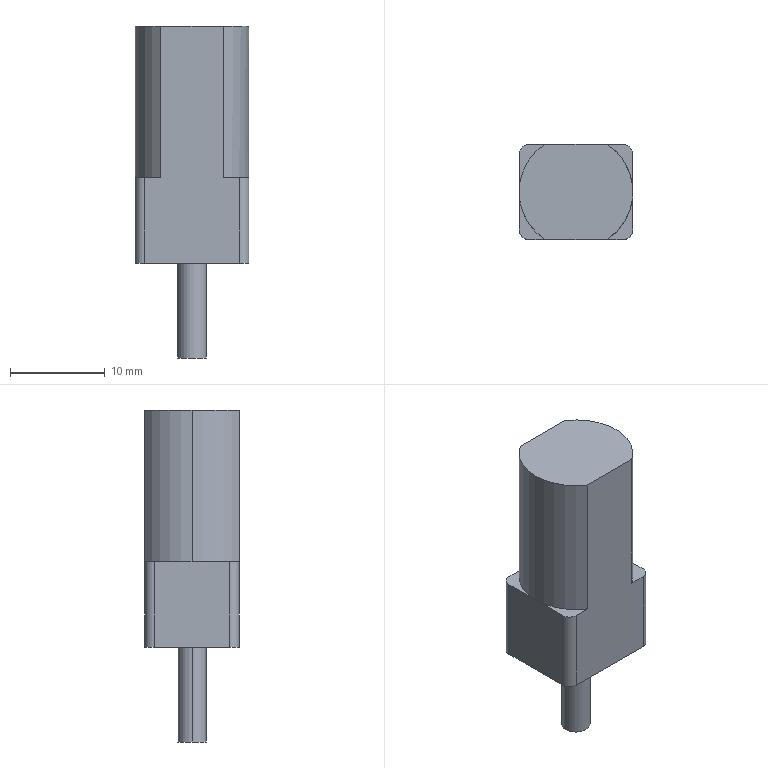Part | STEP file | N201 | 1 solid | 26 faces | box 12 x 10 x 35 mm | volume 2772 mm3 | cylinder 13 | plane 13 | commonest cylinder face diameters 1.6 x4 2 x4 12 x3 3 x2